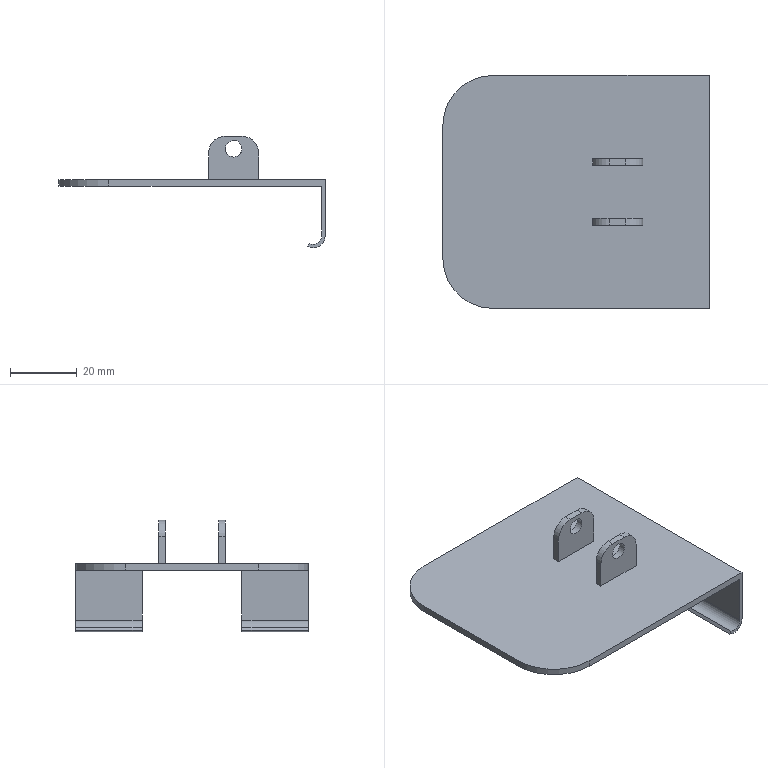Part | NX | features DATUM_CSYS 8, EXTRUDE 7, SKETCH 7, BLEND 2 | 1 solid | 34 faces | box 80 x 70 x 33.5 mm | volume 12516 mm3 | plane 22 | cylinder 12 | commonest cylinder face diameters 5 x4 10 x4 7 x2 30 x2
STEP:
#1=CARTESIAN_POINT('',(22.756,-45.,-24.669));
#2=VERTEX_POINT('',#1);
#3=CARTESIAN_POINT('',(22.756,-25.,-24.669));
#4=VERTEX_POINT('',#3);
#5=CARTESIAN_POINT('',(22.756,-668.,-24.669));
#6=DIRECTION('',(0.,1.,0.));
#7=VECTOR('',#6,1000.);
#8=LINE('',#5,#7);
#9=EDGE_CURVE('',#2,#4,#8,.T.);
#10=ORIENTED_EDGE('',*,*,#9,.T.);
#11=CARTESIAN_POINT('',(22.259,-25.,-25.536));
#12=VERTEX_POINT('',#11);
#13=CARTESIAN_POINT('',(22.756,-25.,-24.669));
#14=DIRECTION('',(-0.4974,0.,-0.8675));
#15=VECTOR('',#14,1000.);
#16=LINE('',#13,#15);
#17=EDGE_CURVE('',#4,#12,#16,.T.);
#18=ORIENTED_EDGE('',*,*,#17,.T.);
#19=CARTESIAN_POINT('',(22.259,-45.,-25.536));
#20=VERTEX_POINT('',#19);
#21=CARTESIAN_POINT('',(22.259,-668.,-25.536));
#22=DIRECTION('',(0.,1.,0.));
#23=VECTOR('',#22,1000.);
#24=LINE('',#21,#23);
#25=EDGE_CURVE('',#20,#12,#24,.T.);
#26=ORIENTED_EDGE('',*,*,#25,.F.);
#27=CARTESIAN_POINT('',(22.756,-45.,-24.669));
#28=DIRECTION('',(-0.4974,0.,-0.8675));
#29=VECTOR('',#28,1000.);
#30=LINE('',#27,#29);
#31=EDGE_CURVE('',#2,#20,#30,.T.);
#32=ORIENTED_EDGE('',*,*,#31,.F.);
#33=EDGE_LOOP('',(#10,#18,#26,#32));
#34=FACE_BOUND('',#33,.T.);
#35=CARTESIAN_POINT('',(22.756,-668.,-24.669));
#36=DIRECTION('',(0.8675,0.,-0.4974));
#37=DIRECTION('',(-0.4974,0.,-0.8675));
#38=AXIS2_PLACEMENT_3D('',#35,#36,#37);
#39=PLANE('',#38);
#40=ADVANCED_FACE('',(#34),#39,.F.);
#41=ORIENTED_EDGE('',*,*,#25,.T.);
#42=CARTESIAN_POINT('',(27.5,-25.,-22.5));
#43=VERTEX_POINT('',#42);
#44=CARTESIAN_POINT('',(24.,-25.,-22.5));
#45=DIRECTION('',(0.,-1.,0.));
#46=DIRECTION('',(0.,0.,-1.));
#47=AXIS2_PLACEMENT_3D('',#44,#45,#46);
#48=CIRCLE('',#47,3.5);
#49=EDGE_CURVE('',#12,#43,#48,.T.);
#50=ORIENTED_EDGE('',*,*,#49,.T.);
#51=CARTESIAN_POINT('',(27.5,-45.,-22.5));
#52=VERTEX_POINT('',#51);
#53=CARTESIAN_POINT('',(27.5,-25.,-22.5));
#54=DIRECTION('',(0.,-1.,0.));
#55=VECTOR('',#54,1000.);
#56=LINE('',#53,#55);
#57=EDGE_CURVE('',#43,#52,#56,.T.);
#58=ORIENTED_EDGE('',*,*,#57,.T.);
#59=CARTESIAN_POINT('',(24.,-45.,-22.5));
#60=DIRECTION('',(0.,-1.,0.));
#61=DIRECTION('',(1.,0.,0.));
#62=AXIS2_PLACEMENT_3D('',#59,#60,#61);
#63=CIRCLE('',#62,3.5);
#64=EDGE_CURVE('',#20,#52,#63,.T.);
#65=ORIENTED_EDGE('',*,*,#64,.F.);
#66=EDGE_LOOP('',(#41,#50,#58,#65));
#67=FACE_BOUND('',#66,.T.);
#68=CARTESIAN_POINT('',(24.,-668.,-22.5));
#69=DIRECTION('',(0.,1.,0.));
#70=DIRECTION('',(-1.,0.,0.));
#71=AXIS2_PLACEMENT_3D('',#68,#69,#70);
#72=CYLINDRICAL_SURFACE('',#71,3.5);
#73=ADVANCED_FACE('',(#67),#72,.T.);
#74=CARTESIAN_POINT('',(26.5,-45.,-22.5));
#75=VERTEX_POINT('',#74);
#76=CARTESIAN_POINT('',(26.5,-25.,-22.5));
#77=VERTEX_POINT('',#76);
#78=CARTESIAN_POINT('',(26.5,-45.,-22.5));
#79=DIRECTION('',(0.,1.,0.));
#80=VECTOR('',#79,1000.);
#81=LINE('',#78,#80);
#82=EDGE_CURVE('',#75,#77,#81,.T.);
#83=ORIENTED_EDGE('',*,*,#82,.T.);
#84=CARTESIAN_POINT('',(24.,-25.,-22.5));
#85=DIRECTION('',(0.,-1.,0.));
#86=DIRECTION('',(0.,0.,-1.));
#87=AXIS2_PLACEMENT_3D('',#84,#85,#86);
#88=CIRCLE('',#87,2.5);
#89=EDGE_CURVE('',#77,#4,#88,.F.);
#90=ORIENTED_EDGE('',*,*,#89,.T.);
#91=ORIENTED_EDGE('',*,*,#9,.F.);
#92=CARTESIAN_POINT('',(24.,-45.,-22.5));
#93=DIRECTION('',(0.,-1.,0.));
#94=DIRECTION('',(1.,0.,0.));
#95=AXIS2_PLACEMENT_3D('',#92,#93,#94);
#96=CIRCLE('',#95,2.5);
#97=EDGE_CURVE('',#75,#2,#96,.F.);
#98=ORIENTED_EDGE('',*,*,#97,.F.);
#99=EDGE_LOOP('',(#83,#90,#91,#98));
#100=FACE_BOUND('',#99,.T.);
#101=CARTESIAN_POINT('',(24.,-668.,-22.5));
#102=DIRECTION('',(0.,1.,0.));
#103=DIRECTION('',(-1.,0.,0.));
#104=AXIS2_PLACEMENT_3D('',#101,#102,#103);
#105=CYLINDRICAL_SURFACE('',#104,2.5);
#106=ADVANCED_FACE('',(#100),#105,.F.);
#107=CARTESIAN_POINT('',(-52.5,-30.,-7.5));
#108=VERTEX_POINT('',#107);
#109=CARTESIAN_POINT('',(-52.5,10.,-7.5));
#110=VERTEX_POINT('',#109);
#111=CARTESIAN_POINT('',(-52.5,-45.,-7.5));
#112=DIRECTION('',(0.,1.,0.));
#113=VECTOR('',#112,1000.);
#114=LINE('',#111,#113);
#115=EDGE_CURVE('',#108,#110,#114,.T.);
#116=ORIENTED_EDGE('',*,*,#115,.T.);
#117=CARTESIAN_POINT('',(-37.5,25.,-7.5));
#118=VERTEX_POINT('',#117);
#119=CARTESIAN_POINT('',(-37.5,10.,-7.5));
#120=DIRECTION('',(0.,0.,1.));
#121=DIRECTION('',(1.,0.,0.));
#122=AXIS2_PLACEMENT_3D('',#119,#120,#121);
#123=CIRCLE('',#122,15.);
#124=EDGE_CURVE('',#110,#118,#123,.F.);
#125=ORIENTED_EDGE('',*,*,#124,.T.);
#126=CARTESIAN_POINT('',(26.5,25.,-7.5));
#127=VERTEX_POINT('',#126);
#128=CARTESIAN_POINT('',(-52.5,25.,-7.5));
#129=DIRECTION('',(1.,0.,0.));
#130=VECTOR('',#129,1000.);
#131=LINE('',#128,#130);
#132=EDGE_CURVE('',#118,#127,#131,.T.);
#133=ORIENTED_EDGE('',*,*,#132,.T.);
#134=CARTESIAN_POINT('',(26.5,5.,-7.5));
#135=VERTEX_POINT('',#134);
#136=CARTESIAN_POINT('',(26.5,5.,-7.5));
#137=DIRECTION('',(0.,1.,0.));
#138=VECTOR('',#137,1000.);
#139=LINE('',#136,#138);
#140=EDGE_CURVE('',#135,#127,#139,.T.);
#141=ORIENTED_EDGE('',*,*,#140,.F.);
#142=CARTESIAN_POINT('',(27.5,5.,-7.5));
#143=VERTEX_POINT('',#142);
#144=CARTESIAN_POINT('',(27.5,5.,-7.5));
#145=DIRECTION('',(-1.,0.,0.));
#146=VECTOR('',#145,1000.);
#147=LINE('',#144,#146);
#148=EDGE_CURVE('',#143,#135,#147,.T.);
#149=ORIENTED_EDGE('',*,*,#148,.F.);
#150=CARTESIAN_POINT('',(27.5,-25.,-7.5));
#151=VERTEX_POINT('',#150);
#152=CARTESIAN_POINT('',(27.5,25.,-7.5));
#153=DIRECTION('',(0.,-1.,0.));
#154=VECTOR('',#153,1000.);
#155=LINE('',#152,#154);
#156=EDGE_CURVE('',#143,#151,#155,.T.);
#157=ORIENTED_EDGE('',*,*,#156,.T.);
#158=CARTESIAN_POINT('',(26.5,-25.,-7.5));
#159=VERTEX_POINT('',#158);
#160=CARTESIAN_POINT('',(26.5,-25.,-7.5));
#161=DIRECTION('',(1.,0.,0.));
#162=VECTOR('',#161,1000.);
#163=LINE('',#160,#162);
#164=EDGE_CURVE('',#159,#151,#163,.T.);
#165=ORIENTED_EDGE('',*,*,#164,.F.);
#166=CARTESIAN_POINT('',(26.5,-45.,-7.5));
#167=VERTEX_POINT('',#166);
#168=CARTESIAN_POINT('',(26.5,-45.,-7.5));
#169=DIRECTION('',(0.,1.,0.));
#170=VECTOR('',#169,1000.);
#171=LINE('',#168,#170);
#172=EDGE_CURVE('',#167,#159,#171,.T.);
#173=ORIENTED_EDGE('',*,*,#172,.F.);
#174=CARTESIAN_POINT('',(-37.5,-45.,-7.5));
#175=VERTEX_POINT('',#174);
#176=CARTESIAN_POINT('',(27.5,-45.,-7.5));
#177=DIRECTION('',(-1.,0.,0.));
#178=VECTOR('',#177,1000.);
#179=LINE('',#176,#178);
#180=EDGE_CURVE('',#167,#175,#179,.T.);
#181=ORIENTED_EDGE('',*,*,#180,.T.);
#182=CARTESIAN_POINT('',(-37.5,-30.,-7.5));
#183=DIRECTION('',(0.,0.,1.));
#184=DIRECTION('',(1.,0.,0.));
#185=AXIS2_PLACEMENT_3D('',#182,#183,#184);
#186=CIRCLE('',#185,15.);
#187=EDGE_CURVE('',#175,#108,#186,.F.);
#188=ORIENTED_EDGE('',*,*,#187,.T.);
#189=EDGE_LOOP('',(#116,#125,#133,#141,#149,#157,#165,#173,#181,#188));
#190=FACE_BOUND('',#189,.T.);
#191=CARTESIAN_POINT('',(-7.5,-20.,-7.5));
#192=DIRECTION('',(0.,0.,1.));
#193=DIRECTION('',(1.,0.,0.));
#194=AXIS2_PLACEMENT_3D('',#191,#192,#193);
#195=PLANE('',#194);
#196=ADVANCED_FACE('',(#190),#195,.F.);
#197=CARTESIAN_POINT('',(-7.5,-20.,2.5));
#198=VERTEX_POINT('',#197);
#199=CARTESIAN_POINT('',(-7.5,-20.,-5.5));
#200=VERTEX_POINT('',#199);
#201=CARTESIAN_POINT('',(-7.5,-20.,7.5));
#202=DIRECTION('',(0.,0.,-1.));
#203=VECTOR('',#202,1000.);
#204=LINE('',#201,#203);
#205=EDGE_CURVE('',#198,#200,#204,.T.);
#206=ORIENTED_EDGE('',*,*,#205,.F.);
#207=CARTESIAN_POINT('',(-7.5,-18.,2.5));
#208=VERTEX_POINT('',#207);
#209=CARTESIAN_POINT('',(-7.5,-20.,2.5));
#210=DIRECTION('',(0.,1.,0.));
#211=VECTOR('',#210,1000.);
#212=LINE('',#209,#211);
#213=EDGE_CURVE('',#198,#208,#212,.T.);
#214=ORIENTED_EDGE('',*,*,#213,.T.);
#215=CARTESIAN_POINT('',(-7.5,-18.,-5.5));
#216=VERTEX_POINT('',#215);
#217=CARTESIAN_POINT('',(-7.5,-18.,7.5));
#218=DIRECTION('',(0.,0.,-1.));
#219=VECTOR('',#218,1000.);
#220=LINE('',#217,#219);
#221=EDGE_CURVE('',#208,#216,#220,.T.);
#222=ORIENTED_EDGE('',*,*,#221,.T.);
#223=CARTESIAN_POINT('',(-7.5,-20.,-5.5));
#224=DIRECTION('',(0.,1.,0.));
#225=VECTOR('',#224,1000.);
#226=LINE('',#223,#225);
#227=EDGE_CURVE('',#216,#200,#226,.F.);
#228=ORIENTED_EDGE('',*,*,#227,.T.);
#229=EDGE_LOOP('',(#206,#214,#222,#228));
#230=FACE_BOUND('',#229,.T.);
#231=CARTESIAN_POINT('',(-7.5,-20.,7.5));
#232=DIRECTION('',(1.,0.,0.));
#233=DIRECTION('',(0.,0.,-1.));
#234=AXIS2_PLACEMENT_3D('',#231,#232,#233);
#235=PLANE('',#234);
#236=ADVANCED_FACE('',(#230),#235,.F.);
#237=CARTESIAN_POINT('',(-7.5,-2.,-5.5));
#238=VERTEX_POINT('',#237);
#239=CARTESIAN_POINT('',(-7.5,-2.,2.5));
#240=VERTEX_POINT('',#239);
#241=CARTESIAN_POINT('',(-7.5,-2.,7.5));
#242=DIRECTION('',(0.,0.,1.));
#243=VECTOR('',#242,1000.);
#244=LINE('',#241,#243);
#245=EDGE_CURVE('',#238,#240,#244,.T.);
#246=ORIENTED_EDGE('',*,*,#245,.T.);
#247=CARTESIAN_POINT('',(-7.5,0.,2.5));
#248=VERTEX_POINT('',#247);
#249=CARTESIAN_POINT('',(-7.5,-20.,2.5));
#250=DIRECTION('',(0.,1.,0.));
#251=VECTOR('',#250,1000.);
#252=LINE('',#249,#251);
#253=EDGE_CURVE('',#240,#248,#252,.T.);
#254=ORIENTED_EDGE('',*,*,#253,.T.);
#255=CARTESIAN_POINT('',(-7.5,0.,-5.5));
#256=VERTEX_POINT('',#255);
#257=CARTESIAN_POINT('',(-7.5,0.,7.5));
#258=DIRECTION('',(0.,0.,-1.));
#259=VECTOR('',#258,1000.);
#260=LINE('',#257,#259);
#261=EDGE_CURVE('',#248,#256,#260,.T.);
#262=ORIENTED_EDGE('',*,*,#261,.T.);
#263=CARTESIAN_POINT('',(-7.5,-20.,-5.5));
#264=DIRECTION('',(0.,1.,0.));
#265=VECTOR('',#264,1000.);
#266=LINE('',#263,#265);
#267=EDGE_CURVE('',#256,#238,#266,.F.);
#268=ORIENTED_EDGE('',*,*,#267,.T.);
#269=EDGE_LOOP('',(#246,#254,#262,#268));
#270=FACE_BOUND('',#269,.T.);
#271=CARTESIAN_POINT('',(-7.5,-20.,7.5));
#272=DIRECTION('',(1.,0.,0.));
#273=DIRECTION('',(0.,0.,-1.));
#274=AXIS2_PLACEMENT_3D('',#271,#272,#273);
#275=PLANE('',#274);
#276=ADVANCED_FACE('',(#270),#275,.F.);
#277=CARTESIAN_POINT('',(7.5,0.,-5.5));
#278=VERTEX_POINT('',#277);
#279=CARTESIAN_POINT('',(7.5,0.,2.5));
#280=VERTEX_POINT('',#279);
#281=CARTESIAN_POINT('',(7.5,0.,-7.5));
#282=DIRECTION('',(0.,0.,1.));
#283=VECTOR('',#282,1000.);
#284=LINE('',#281,#283);
#285=EDGE_CURVE('',#278,#280,#284,.T.);
#286=ORIENTED_EDGE('',*,*,#285,.T.);
#287=CARTESIAN_POINT('',(7.5,-2.,2.5));
#288=VERTEX_POINT('',#287);
#289=CARTESIAN_POINT('',(7.5,-20.,2.5));
#290=DIRECTION('',(0.,1.,0.));
#291=VECTOR('',#290,1000.);
#292=LINE('',#289,#291);
#293=EDGE_CURVE('',#280,#288,#292,.F.);
#294=ORIENTED_EDGE('',*,*,#293,.T.);
#295=CARTESIAN_POINT('',(7.5,-2.,-5.5));
#296=VERTEX_POINT('',#295);
#297=CARTESIAN_POINT('',(7.5,-2.,-7.5));
#298=DIRECTION('',(0.,0.,-1.));
#299=VECTOR('',#298,1000.);
#300=LINE('',#297,#299);
#301=EDGE_CURVE('',#288,#296,#300,.T.);
#302=ORIENTED_EDGE('',*,*,#301,.T.);
#303=CARTESIAN_POINT('',(7.5,-20.,-5.5));
#304=DIRECTION('',(0.,-1.,0.));
#305=VECTOR('',#304,1000.);
#306=LINE('',#303,#305);
#307=EDGE_CURVE('',#296,#278,#306,.F.);
#308=ORIENTED_EDGE('',*,*,#307,.T.);
#309=EDGE_LOOP('',(#286,#294,#302,#308));
#310=FACE_BOUND('',#309,.T.);
#311=CARTESIAN_POINT('',(7.5,-20.,-7.5));
#312=DIRECTION('',(-1.,0.,0.));
#313=DIRECTION('',(0.,0.,1.));
#314=AXIS2_PLACEMENT_3D('',#311,#312,#313);
#315=PLANE('',#314);
#316=ADVANCED_FACE('',(#310),#315,.F.);
#317=CARTESIAN_POINT('',(7.5,-18.,-5.5));
#318=VERTEX_POINT('',#317);
#319=CARTESIAN_POINT('',(7.5,-18.,2.5));
#320=VERTEX_POINT('',#319);
#321=CARTESIAN_POINT('',(7.5,-18.,-7.5));
#322=DIRECTION('',(0.,0.,1.));
#323=VECTOR('',#322,1000.);
#324=LINE('',#321,#323);
#325=EDGE_CURVE('',#318,#320,#324,.T.);
#326=ORIENTED_EDGE('',*,*,#325,.T.);
#327=CARTESIAN_POINT('',(7.5,-20.,2.5));
#328=VERTEX_POINT('',#327);
#329=CARTESIAN_POINT('',(7.5,-20.,2.5));
#330=DIRECTION('',(0.,1.,0.));
#331=VECTOR('',#330,1000.);
#332=LINE('',#329,#331);
#333=EDGE_CURVE('',#320,#328,#332,.F.);
#334=ORIENTED_EDGE('',*,*,#333,.T.);
#335=CARTESIAN_POINT('',(7.5,-20.,-5.5));
#336=VERTEX_POINT('',#335);
#337=CARTESIAN_POINT('',(7.5,-20.,-7.5));
#338=DIRECTION('',(0.,0.,1.));
#339=VECTOR('',#338,1000.);
#340=LINE('',#337,#339);
#341=EDGE_CURVE('',#336,#328,#340,.T.);
#342=ORIENTED_EDGE('',*,*,#341,.F.);
#343=CARTESIAN_POINT('',(7.5,-20.,-5.5));
#344=DIRECTION('',(0.,-1.,0.));
#345=VECTOR('',#344,1000.);
#346=LINE('',#343,#345);
#347=EDGE_CURVE('',#336,#318,#346,.F.);
#348=ORIENTED_EDGE('',*,*,#347,.T.);
#349=EDGE_LOOP('',(#326,#334,#342,#348));
#350=FACE_BOUND('',#349,.T.);
#351=CARTESIAN_POINT('',(7.5,-20.,-7.5));
#352=DIRECTION('',(-1.,0.,0.));
#353=DIRECTION('',(0.,0.,1.));
#354=AXIS2_PLACEMENT_3D('',#351,#352,#353);
#355=PLANE('',#354);
#356=ADVANCED_FACE('',(#350),#355,.F.);
#357=CARTESIAN_POINT('',(0.,-20.,1.25));
#358=VERTEX_POINT('',#357);
#359=CARTESIAN_POINT('',(0.,-20.,3.75));
#360=DIRECTION('',(0.,-1.,0.));
#361=DIRECTION('',(0.,0.,-1.));
#362=AXIS2_PLACEMENT_3D('',#359,#360,#361);
#363=CIRCLE('',#362,2.5);
#364=EDGE_CURVE('',#358,#358,#363,.T.);
#365=ORIENTED_EDGE('',*,*,#364,.F.);
#366=EDGE_LOOP('',(#365));
#367=FACE_BOUND('',#366,.T.);
#368=CARTESIAN_POINT('',(2.5,-20.,7.5));
#369=VERTEX_POINT('',#368);
#370=CARTESIAN_POINT('',(-2.5,-20.,7.5));
#371=VERTEX_POINT('',#370);
#372=CARTESIAN_POINT('',(7.5,-20.,7.5));
#373=DIRECTION('',(-1.,0.,0.));
#374=VECTOR('',#373,1000.);
#375=LINE('',#372,#374);
#376=EDGE_CURVE('',#369,#371,#375,.T.);
#377=ORIENTED_EDGE('',*,*,#376,.T.);
#378=CARTESIAN_POINT('',(-2.5,-20.,2.5));
#379=DIRECTION('',(0.,-1.,0.));
#380=DIRECTION('',(0.,0.,-1.));
#381=AXIS2_PLACEMENT_3D('',#378,#379,#380);
#382=CIRCLE('',#381,5.);
#383=EDGE_CURVE('',#371,#198,#382,.T.);
#384=ORIENTED_EDGE('',*,*,#383,.T.);
#385=ORIENTED_EDGE('',*,*,#205,.T.);
#386=CARTESIAN_POINT('',(0.,-20.,-5.5));
#387=DIRECTION('',(1.,0.,0.));
#388=VECTOR('',#387,1000.);
#389=LINE('',#386,#388);
#390=EDGE_CURVE('',#200,#336,#389,.T.);
#391=ORIENTED_EDGE('',*,*,#390,.T.);
#392=ORIENTED_EDGE('',*,*,#341,.T.);
#393=CARTESIAN_POINT('',(2.5,-20.,2.5));
#394=DIRECTION('',(0.,-1.,0.));
#395=DIRECTION('',(0.,0.,-1.));
#396=AXIS2_PLACEMENT_3D('',#393,#394,#395);
#397=CIRCLE('',#396,5.);
#398=EDGE_CURVE('',#328,#369,#397,.T.);
#399=ORIENTED_EDGE('',*,*,#398,.T.);
#400=EDGE_LOOP('',(#377,#384,#385,#391,#392,#399));
#401=FACE_BOUND('',#400,.T.);
#402=CARTESIAN_POINT('',(0.,-20.,0.));
#403=DIRECTION('',(0.,-1.,0.));
#404=DIRECTION('',(0.,0.,-1.));
#405=AXIS2_PLACEMENT_3D('',#402,#403,#404);
#406=PLANE('',#405);
#407=ADVANCED_FACE('',(#367,#401),#406,.T.);
#408=CARTESIAN_POINT('',(-2.5,0.,3.75));
#409=VERTEX_POINT('',#408);
#410=CARTESIAN_POINT('',(0.,0.,3.75));
#411=DIRECTION('',(0.,1.,0.));
#412=DIRECTION('',(-1.,0.,0.));
#413=AXIS2_PLACEMENT_3D('',#410,#411,#412);
#414=CIRCLE('',#413,2.5);
#415=EDGE_CURVE('',#409,#409,#414,.T.);
#416=ORIENTED_EDGE('',*,*,#415,.F.);
#417=EDGE_LOOP('',(#416));
#418=FACE_BOUND('',#417,.T.);
#419=CARTESIAN_POINT('',(2.5,0.,7.5));
#420=VERTEX_POINT('',#419);
#421=CARTESIAN_POINT('',(-2.5,0.,7.5));
#422=VERTEX_POINT('',#421);
#423=CARTESIAN_POINT('',(7.5,0.,7.5));
#424=DIRECTION('',(-1.,0.,0.));
#425=VECTOR('',#424,1000.);
#426=LINE('',#423,#425);
#427=EDGE_CURVE('',#420,#422,#426,.T.);
#428=ORIENTED_EDGE('',*,*,#427,.F.);
#429=CARTESIAN_POINT('',(2.5,0.,2.5));
#430=DIRECTION('',(0.,-1.,0.));
#431=DIRECTION('',(0.,0.,-1.));
#432=AXIS2_PLACEMENT_3D('',#429,#430,#431);
#433=CIRCLE('',#432,5.);
#434=EDGE_CURVE('',#420,#280,#433,.F.);
#435=ORIENTED_EDGE('',*,*,#434,.T.);
#436=ORIENTED_EDGE('',*,*,#285,.F.);
#437=CARTESIAN_POINT('',(0.,0.,-5.5));
#438=DIRECTION('',(1.,0.,0.));
#439=VECTOR('',#438,1000.);
#440=LINE('',#437,#439);
#441=EDGE_CURVE('',#256,#278,#440,.T.);
#442=ORIENTED_EDGE('',*,*,#441,.F.);
#443=ORIENTED_EDGE('',*,*,#261,.F.);
#444=CARTESIAN_POINT('',(-2.5,0.,2.5));
#445=DIRECTION('',(0.,-1.,0.));
#446=DIRECTION('',(0.,0.,-1.));
#447=AXIS2_PLACEMENT_3D('',#444,#445,#446);
#448=CIRCLE('',#447,5.);
#449=EDGE_CURVE('',#248,#422,#448,.F.);
#450=ORIENTED_EDGE('',*,*,#449,.T.);
#451=EDGE_LOOP('',(#428,#435,#436,#442,#443,#450));
#452=FACE_BOUND('',#451,.T.);
#453=CARTESIAN_POINT('',(0.,0.,0.));
#454=DIRECTION('',(0.,-1.,0.));
#455=DIRECTION('',(0.,0.,-1.));
#456=AXIS2_PLACEMENT_3D('',#453,#454,#455);
#457=PLANE('',#456);
#458=ADVANCED_FACE('',(#418,#452),#457,.F.);
#459=CARTESIAN_POINT('',(-2.5,-2.,7.5));
#460=VERTEX_POINT('',#459);
#461=CARTESIAN_POINT('',(2.5,-2.,7.5));
#462=VERTEX_POINT('',#461);
#463=CARTESIAN_POINT('',(7.5,-2.,7.5));
#464=DIRECTION('',(1.,0.,0.));
#465=VECTOR('',#464,1000.);
#466=LINE('',#463,#465);
#467=EDGE_CURVE('',#460,#462,#466,.T.);
#468=ORIENTED_EDGE('',*,*,#467,.T.);
#469=CARTESIAN_POINT('',(2.5,-20.,7.5));
#470=DIRECTION('',(0.,1.,0.));
#471=VECTOR('',#470,1000.);
#472=LINE('',#469,#471);
#473=EDGE_CURVE('',#462,#420,#472,.T.);
#474=ORIENTED_EDGE('',*,*,#473,.T.);
#475=ORIENTED_EDGE('',*,*,#427,.T.);
#476=CARTESIAN_POINT('',(-2.5,-20.,7.5));
#477=DIRECTION('',(0.,1.,0.));
#478=VECTOR('',#477,1000.);
#479=LINE('',#476,#478);
#480=EDGE_CURVE('',#422,#460,#479,.F.);
#481=ORIENTED_EDGE('',*,*,#480,.T.);
#482=EDGE_LOOP('',(#468,#474,#475,#481));
#483=FACE_BOUND('',#482,.T.);
#484=CARTESIAN_POINT('',(7.5,-20.,7.5));
#485=DIRECTION('',(0.,0.,-1.));
#486=DIRECTION('',(-1.,0.,0.));
#487=AXIS2_PLACEMENT_3D('',#484,#485,#486);
#488=PLANE('',#487);
#489=ADVANCED_FACE('',(#483),#488,.F.);
#490=CARTESIAN_POINT('',(2.5,-18.,7.5));
#491=VERTEX_POINT('',#490);
#492=CARTESIAN_POINT('',(-2.5,-18.,7.5));
#493=VERTEX_POINT('',#492);
#494=CARTESIAN_POINT('',(7.5,-18.,7.5));
#495=DIRECTION('',(-1.,0.,0.));
#496=VECTOR('',#495,1000.);
#497=LINE('',#494,#496);
#498=EDGE_CURVE('',#491,#493,#497,.T.);
#499=ORIENTED_EDGE('',*,*,#498,.T.);
#500=CARTESIAN_POINT('',(-2.5,-20.,7.5));
#501=DIRECTION('',(0.,1.,0.));
#502=VECTOR('',#501,1000.);
#503=LINE('',#500,#502);
#504=EDGE_CURVE('',#493,#371,#503,.F.);
#505=ORIENTED_EDGE('',*,*,#504,.T.);
#506=ORIENTED_EDGE('',*,*,#376,.F.);
#507=CARTESIAN_POINT('',(2.5,-20.,7.5));
#508=DIRECTION('',(0.,1.,0.));
#509=VECTOR('',#508,1000.);
#510=LINE('',#507,#509);
#511=EDGE_CURVE('',#369,#491,#510,.T.);
#512=ORIENTED_EDGE('',*,*,#511,.T.);
#513=EDGE_LOOP('',(#499,#505,#506,#512));
#514=FACE_BOUND('',#513,.T.);
#515=CARTESIAN_POINT('',(7.5,-20.,7.5));
#516=DIRECTION('',(0.,0.,-1.));
#517=DIRECTION('',(-1.,0.,0.));
#518=AXIS2_PLACEMENT_3D('',#515,#516,#517);
#519=PLANE('',#518);
#520=ADVANCED_FACE('',(#514),#519,.F.);
#521=CARTESIAN_POINT('',(-23.,-2.,-5.5));
#522=DIRECTION('',(1.,0.,0.));
#523=VECTOR('',#522,1000.);
#524=LINE('',#521,#523);
#525=EDGE_CURVE('',#296,#238,#524,.F.);
#526=ORIENTED_EDGE('',*,*,#525,.T.);
#527=ORIENTED_EDGE('',*,*,#267,.F.);
#528=ORIENTED_EDGE('',*,*,#441,.T.);
#529=ORIENTED_EDGE('',*,*,#307,.F.);
#530=EDGE_LOOP('',(#526,#527,#528,#529));
#531=FACE_BOUND('',#530,.T.);
#532=CARTESIAN_POINT('',(21.,-18.,-5.5));
#533=DIRECTION('',(-1.,0.,0.));
#534=VECTOR('',#533,1000.);
#535=LINE('',#532,#534);
#536=EDGE_CURVE('',#216,#318,#535,.F.);
#537=ORIENTED_EDGE('',*,*,#536,.T.);
#538=ORIENTED_EDGE('',*,*,#347,.F.);
#539=ORIENTED_EDGE('',*,*,#390,.F.);
#540=ORIENTED_EDGE('',*,*,#227,.F.);
#541=EDGE_LOOP('',(#537,#538,#539,#540));
#542=FACE_BOUND('',#541,.T.);
#543=CARTESIAN_POINT('',(-37.5,25.,-5.5));
#544=VERTEX_POINT('',#543);
#545=CARTESIAN_POINT('',(27.5,25.,-5.5));
#546=VERTEX_POINT('',#545);
#547=CARTESIAN_POINT('',(-52.5,25.,-5.5));
#548=DIRECTION('',(1.,0.,0.));
#549=VECTOR('',#548,1000.);
#550=LINE('',#547,#549);
#551=EDGE_CURVE('',#544,#546,#550,.T.);
#552=ORIENTED_EDGE('',*,*,#551,.F.);
#553=CARTESIAN_POINT('',(-52.5,10.,-5.5));
#554=VERTEX_POINT('',#553);
#555=CARTESIAN_POINT('',(-37.5,10.,-5.5));
#556=DIRECTION('',(0.,0.,-1.));
#557=DIRECTION('',(-1.,0.,0.));
#558=AXIS2_PLACEMENT_3D('',#555,#556,#557);
#559=CIRCLE('',#558,15.);
#560=EDGE_CURVE('',#544,#554,#559,.F.);
#561=ORIENTED_EDGE('',*,*,#560,.T.);
#562=CARTESIAN_POINT('',(-52.5,-30.,-5.5));
#563=VERTEX_POINT('',#562);
#564=CARTESIAN_POINT('',(-52.5,-45.,-5.5));
#565=DIRECTION('',(0.,1.,0.));
#566=VECTOR('',#565,1000.);
#567=LINE('',#564,#566);
#568=EDGE_CURVE('',#563,#554,#567,.T.);
#569=ORIENTED_EDGE('',*,*,#568,.F.);
#570=CARTESIAN_POINT('',(-37.5,-45.,-5.5));
#571=VERTEX_POINT('',#570);
#572=CARTESIAN_POINT('',(-37.5,-30.,-5.5));
#573=DIRECTION('',(0.,0.,-1.));
#574=DIRECTION('',(-1.,0.,0.));
#575=AXIS2_PLACEMENT_3D('',#572,#573,#574);
#576=CIRCLE('',#575,15.);
#577=EDGE_CURVE('',#563,#571,#576,.F.);
#578=ORIENTED_EDGE('',*,*,#577,.T.);
#579=CARTESIAN_POINT('',(27.5,-45.,-5.5));
#580=VERTEX_POINT('',#579);
#581=CARTESIAN_POINT('',(27.5,-45.,-5.5));
#582=DIRECTION('',(-1.,0.,0.));
#583=VECTOR('',#582,1000.);
#584=LINE('',#581,#583);
#585=EDGE_CURVE('',#580,#571,#584,.T.);
#586=ORIENTED_EDGE('',*,*,#585,.F.);
#587=CARTESIAN_POINT('',(27.5,25.,-5.5));
#588=DIRECTION('',(0.,-1.,0.));
#589=VECTOR('',#588,1000.);
#590=LINE('',#587,#589);
#591=EDGE_CURVE('',#546,#580,#590,.T.);
#592=ORIENTED_EDGE('',*,*,#591,.F.);
#593=EDGE_LOOP('',(#552,#561,#569,#578,#586,#592));
#594=FACE_BOUND('',#593,.T.);
#595=CARTESIAN_POINT('',(0.,0.,-5.5));
#596=DIRECTION('',(0.,0.,-1.));
#597=DIRECTION('',(-1.,0.,0.));
#598=AXIS2_PLACEMENT_3D('',#595,#596,#597);
#599=PLANE('',#598);
#600=ADVANCED_FACE('',(#531,#542,#594),#599,.F.);
#601=CARTESIAN_POINT('',(-2.5,-2.,3.75));
#602=VERTEX_POINT('',#601);
#603=CARTESIAN_POINT('',(0.,-2.,3.75));
#604=DIRECTION('',(0.,1.,0.));
#605=DIRECTION('',(-1.,0.,0.));
#606=AXIS2_PLACEMENT_3D('',#603,#604,#605);
#607=CIRCLE('',#606,2.5);
#608=EDGE_CURVE('',#602,#602,#607,.T.);
#609=ORIENTED_EDGE('',*,*,#608,.T.);
#610=EDGE_LOOP('',(#609));
#611=FACE_BOUND('',#610,.T.);
#612=ORIENTED_EDGE('',*,*,#301,.F.);
#613=CARTESIAN_POINT('',(2.5,-2.,2.5));
#614=DIRECTION('',(0.,1.,0.));
#615=DIRECTION('',(-1.,0.,0.));
#616=AXIS2_PLACEMENT_3D('',#613,#614,#615);
#617=CIRCLE('',#616,5.);
#618=EDGE_CURVE('',#288,#462,#617,.F.);
#619=ORIENTED_EDGE('',*,*,#618,.T.);
#620=ORIENTED_EDGE('',*,*,#467,.F.);
#621=CARTESIAN_POINT('',(-2.5,-2.,2.5));
#622=DIRECTION('',(0.,1.,0.));
#623=DIRECTION('',(-1.,0.,0.));
#624=AXIS2_PLACEMENT_3D('',#621,#622,#623);
#625=CIRCLE('',#624,5.);
#626=EDGE_CURVE('',#460,#240,#625,.F.);
#627=ORIENTED_EDGE('',*,*,#626,.T.);
#628=ORIENTED_EDGE('',*,*,#245,.F.);
#629=ORIENTED_EDGE('',*,*,#525,.F.);
#630=EDGE_LOOP('',(#612,#619,#620,#627,#628,#629));
#631=FACE_BOUND('',#630,.T.);
#632=CARTESIAN_POINT('',(-23.,-2.,10.5));
#633=DIRECTION('',(0.,1.,0.));
#634=DIRECTION('',(-1.,0.,0.));
#635=AXIS2_PLACEMENT_3D('',#632,#633,#634);
#636=PLANE('',#635);
#637=ADVANCED_FACE('',(#611,#631),#636,.F.);
#638=CARTESIAN_POINT('',(2.5,-18.,3.75));
#639=VERTEX_POINT('',#638);
#640=CARTESIAN_POINT('',(0.,-18.,3.75));
#641=DIRECTION('',(0.,-1.,0.));
#642=DIRECTION('',(1.,0.,0.));
#643=AXIS2_PLACEMENT_3D('',#640,#641,#642);
#644=CIRCLE('',#643,2.5);
#645=EDGE_CURVE('',#639,#639,#644,.T.);
#646=ORIENTED_EDGE('',*,*,#645,.T.);
#647=EDGE_LOOP('',(#646));
#648=FACE_BOUND('',#647,.T.);
#649=ORIENTED_EDGE('',*,*,#221,.F.);
#650=CARTESIAN_POINT('',(-2.5,-18.,2.5));
#651=DIRECTION('',(0.,-1.,0.));
#652=DIRECTION('',(1.,0.,0.));
#653=AXIS2_PLACEMENT_3D('',#650,#651,#652);
#654=CIRCLE('',#653,5.);
#655=EDGE_CURVE('',#208,#493,#654,.F.);
#656=ORIENTED_EDGE('',*,*,#655,.T.);
#657=ORIENTED_EDGE('',*,*,#498,.F.);
#658=CARTESIAN_POINT('',(2.5,-18.,2.5));
#659=DIRECTION('',(0.,-1.,0.));
#660=DIRECTION('',(1.,0.,0.));
#661=AXIS2_PLACEMENT_3D('',#658,#659,#660);
#662=CIRCLE('',#661,5.);
#663=EDGE_CURVE('',#491,#320,#662,.F.);
#664=ORIENTED_EDGE('',*,*,#663,.T.);
#665=ORIENTED_EDGE('',*,*,#325,.F.);
#666=ORIENTED_EDGE('',*,*,#536,.F.);
#667=EDGE_LOOP('',(#649,#656,#657,#664,#665,#666));
#668=FACE_BOUND('',#667,.T.);
#669=CARTESIAN_POINT('',(21.,-18.,10.5));
#670=DIRECTION('',(0.,-1.,0.));
#671=DIRECTION('',(1.,0.,0.));
#672=AXIS2_PLACEMENT_3D('',#669,#670,#671);
#673=PLANE('',#672);
#674=ADVANCED_FACE('',(#648,#668),#673,.F.);
#675=ORIENTED_EDGE('',*,*,#568,.T.);
#676=CARTESIAN_POINT('',(-52.5,10.,-5.5));
#677=DIRECTION('',(0.,0.,-1.));
#678=VECTOR('',#677,1000.);
#679=LINE('',#676,#678);
#680=EDGE_CURVE('',#554,#110,#679,.T.);
#681=ORIENTED_EDGE('',*,*,#680,.T.);
#682=ORIENTED_EDGE('',*,*,#115,.F.);
#683=CARTESIAN_POINT('',(-52.5,-30.,-5.5));
#684=DIRECTION('',(0.,0.,-1.));
#685=VECTOR('',#684,1000.);
#686=LINE('',#683,#685);
#687=EDGE_CURVE('',#108,#563,#686,.F.);
#688=ORIENTED_EDGE('',*,*,#687,.T.);
#689=EDGE_LOOP('',(#675,#681,#682,#688));
#690=FACE_BOUND('',#689,.T.);
#691=CARTESIAN_POINT('',(-52.5,-45.,-5.5));
#692=DIRECTION('',(-1.,0.,0.));
#693=DIRECTION('',(0.,-1.,0.));
#694=AXIS2_PLACEMENT_3D('',#691,#692,#693);
#695=PLANE('',#694);
#696=ADVANCED_FACE('',(#690),#695,.T.);
#697=ORIENTED_EDGE('',*,*,#132,.F.);
#698=CARTESIAN_POINT('',(-37.5,25.,-5.5));
#699=DIRECTION('',(0.,0.,-1.));
#700=VECTOR('',#699,1000.);
#701=LINE('',#698,#700);
#702=EDGE_CURVE('',#118,#544,#701,.F.);
#703=ORIENTED_EDGE('',*,*,#702,.T.);
#704=ORIENTED_EDGE('',*,*,#551,.T.);
#705=CARTESIAN_POINT('',(27.5,25.,-22.5));
#706=VERTEX_POINT('',#705);
#707=CARTESIAN_POINT('',(27.5,25.,-5.5));
#708=DIRECTION('',(0.,0.,-1.));
#709=VECTOR('',#708,1000.);
#710=LINE('',#707,#709);
#711=EDGE_CURVE('',#546,#706,#710,.T.);
#712=ORIENTED_EDGE('',*,*,#711,.T.);
#713=CARTESIAN_POINT('',(22.259,25.,-25.536));
#714=VERTEX_POINT('',#713);
#715=CARTESIAN_POINT('',(24.,25.,-22.5));
#716=DIRECTION('',(0.,-1.,0.));
#717=DIRECTION('',(0.,0.,-1.));
#718=AXIS2_PLACEMENT_3D('',#715,#716,#717);
#719=CIRCLE('',#718,3.5);
#720=EDGE_CURVE('',#714,#706,#719,.T.);
#721=ORIENTED_EDGE('',*,*,#720,.F.);
#722=CARTESIAN_POINT('',(22.756,25.,-24.669));
#723=VERTEX_POINT('',#722);
#724=CARTESIAN_POINT('',(22.756,25.,-24.669));
#725=DIRECTION('',(-0.4974,0.,-0.8675));
#726=VECTOR('',#725,1000.);
#727=LINE('',#724,#726);
#728=EDGE_CURVE('',#723,#714,#727,.T.);
#729=ORIENTED_EDGE('',*,*,#728,.F.);
#730=CARTESIAN_POINT('',(26.5,25.,-22.5));
#731=VERTEX_POINT('',#730);
#732=CARTESIAN_POINT('',(24.,25.,-22.5));
#733=DIRECTION('',(0.,1.,0.));
#734=DIRECTION('',(0.,0.,-1.));
#735=AXIS2_PLACEMENT_3D('',#732,#733,#734);
#736=CIRCLE('',#735,2.5);
#737=EDGE_CURVE('',#731,#723,#736,.T.);
#738=ORIENTED_EDGE('',*,*,#737,.F.);
#739=CARTESIAN_POINT('',(26.5,25.,-22.5));
#740=DIRECTION('',(0.,0.,1.));
#741=VECTOR('',#740,1000.);
#742=LINE('',#739,#741);
#743=EDGE_CURVE('',#731,#127,#742,.T.);
#744=ORIENTED_EDGE('',*,*,#743,.T.);
#745=EDGE_LOOP('',(#697,#703,#704,#712,#721,#729,#738,#744));
#746=FACE_BOUND('',#745,.T.);
#747=CARTESIAN_POINT('',(-52.5,25.,-5.5));
#748=DIRECTION('',(0.,1.,0.));
#749=DIRECTION('',(-1.,0.,0.));
#750=AXIS2_PLACEMENT_3D('',#747,#748,#749);
#751=PLANE('',#750);
#752=ADVANCED_FACE('',(#746),#751,.T.);
#753=ORIENTED_EDGE('',*,*,#156,.F.);
#754=CARTESIAN_POINT('',(27.5,5.,-22.5));
#755=VERTEX_POINT('',#754);
#756=CARTESIAN_POINT('',(27.5,5.,-22.5));
#757=DIRECTION('',(0.,0.,1.));
#758=VECTOR('',#757,1000.);
#759=LINE('',#756,#758);
#760=EDGE_CURVE('',#755,#143,#759,.T.);
#761=ORIENTED_EDGE('',*,*,#760,.F.);
#762=CARTESIAN_POINT('',(27.5,25.,-22.5));
#763=DIRECTION('',(0.,-1.,0.));
#764=VECTOR('',#763,1000.);
#765=LINE('',#762,#764);
#766=EDGE_CURVE('',#706,#755,#765,.T.);
#767=ORIENTED_EDGE('',*,*,#766,.F.);
#768=ORIENTED_EDGE('',*,*,#711,.F.);
#769=ORIENTED_EDGE('',*,*,#591,.T.);
#770=CARTESIAN_POINT('',(27.5,-45.,-5.5));
#771=DIRECTION('',(0.,0.,-1.));
#772=VECTOR('',#771,1000.);
#773=LINE('',#770,#772);
#774=EDGE_CURVE('',#580,#52,#773,.T.);
#775=ORIENTED_EDGE('',*,*,#774,.T.);
#776=ORIENTED_EDGE('',*,*,#57,.F.);
#777=CARTESIAN_POINT('',(27.5,-25.,-22.5));
#778=DIRECTION('',(0.,0.,1.));
#779=VECTOR('',#778,1000.);
#780=LINE('',#777,#779);
#781=EDGE_CURVE('',#43,#151,#780,.T.);
#782=ORIENTED_EDGE('',*,*,#781,.T.);
#783=EDGE_LOOP('',(#753,#761,#767,#768,#769,#775,#776,#782));
#784=FACE_BOUND('',#783,.T.);
#785=CARTESIAN_POINT('',(27.5,25.,-5.5));
#786=DIRECTION('',(1.,0.,0.));
#787=DIRECTION('',(0.,1.,0.));
#788=AXIS2_PLACEMENT_3D('',#785,#786,#787);
#789=PLANE('',#788);
#790=ADVANCED_FACE('',(#784),#789,.T.);
#791=ORIENTED_EDGE('',*,*,#585,.T.);
#792=CARTESIAN_POINT('',(-37.5,-45.,-5.5));
#793=DIRECTION('',(0.,0.,-1.));
#794=VECTOR('',#793,1000.);
#795=LINE('',#792,#794);
#796=EDGE_CURVE('',#571,#175,#795,.T.);
#797=ORIENTED_EDGE('',*,*,#796,.T.);
#798=ORIENTED_EDGE('',*,*,#180,.F.);
#799=CARTESIAN_POINT('',(26.5,-45.,-22.5));
#800=DIRECTION('',(0.,0.,1.));
#801=VECTOR('',#800,1000.);
#802=LINE('',#799,#801);
#803=EDGE_CURVE('',#75,#167,#802,.T.);
#804=ORIENTED_EDGE('',*,*,#803,.F.);
#805=ORIENTED_EDGE('',*,*,#97,.T.);
#806=ORIENTED_EDGE('',*,*,#31,.T.);
#807=ORIENTED_EDGE('',*,*,#64,.T.);
#808=ORIENTED_EDGE('',*,*,#774,.F.);
#809=EDGE_LOOP('',(#791,#797,#798,#804,#805,#806,#807,#808));
#810=FACE_BOUND('',#809,.T.);
#811=CARTESIAN_POINT('',(27.5,-45.,-5.5));
#812=DIRECTION('',(0.,-1.,0.));
#813=DIRECTION('',(1.,0.,0.));
#814=AXIS2_PLACEMENT_3D('',#811,#812,#813);
#815=PLANE('',#814);
#816=ADVANCED_FACE('',(#810),#815,.T.);
#817=ORIENTED_EDGE('',*,*,#172,.T.);
#818=CARTESIAN_POINT('',(26.5,-25.,-22.5));
#819=DIRECTION('',(0.,0.,1.));
#820=VECTOR('',#819,1000.);
#821=LINE('',#818,#820);
#822=EDGE_CURVE('',#77,#159,#821,.T.);
#823=ORIENTED_EDGE('',*,*,#822,.F.);
#824=ORIENTED_EDGE('',*,*,#82,.F.);
#825=ORIENTED_EDGE('',*,*,#803,.T.);
#826=EDGE_LOOP('',(#817,#823,#824,#825));
#827=FACE_BOUND('',#826,.T.);
#828=CARTESIAN_POINT('',(26.5,-45.,-22.5));
#829=DIRECTION('',(1.,0.,0.));
#830=DIRECTION('',(0.,1.,0.));
#831=AXIS2_PLACEMENT_3D('',#828,#829,#830);
#832=PLANE('',#831);
#833=ADVANCED_FACE('',(#827),#832,.F.);
#834=ORIENTED_EDGE('',*,*,#164,.T.);
#835=ORIENTED_EDGE('',*,*,#781,.F.);
#836=ORIENTED_EDGE('',*,*,#49,.F.);
#837=ORIENTED_EDGE('',*,*,#17,.F.);
#838=ORIENTED_EDGE('',*,*,#89,.F.);
#839=ORIENTED_EDGE('',*,*,#822,.T.);
#840=EDGE_LOOP('',(#834,#835,#836,#837,#838,#839));
#841=FACE_BOUND('',#840,.T.);
#842=CARTESIAN_POINT('',(26.5,-25.,-22.5));
#843=DIRECTION('',(0.,-1.,0.));
#844=DIRECTION('',(1.,0.,0.));
#845=AXIS2_PLACEMENT_3D('',#842,#843,#844);
#846=PLANE('',#845);
#847=ADVANCED_FACE('',(#841),#846,.F.);
#848=ORIENTED_EDGE('',*,*,#140,.T.);
#849=ORIENTED_EDGE('',*,*,#743,.F.);
#850=CARTESIAN_POINT('',(26.5,5.,-22.5));
#851=VERTEX_POINT('',#850);
#852=CARTESIAN_POINT('',(26.5,5.,-22.5));
#853=DIRECTION('',(0.,1.,0.));
#854=VECTOR('',#853,1000.);
#855=LINE('',#852,#854);
#856=EDGE_CURVE('',#851,#731,#855,.T.);
#857=ORIENTED_EDGE('',*,*,#856,.F.);
#858=CARTESIAN_POINT('',(26.5,5.,-22.5));
#859=DIRECTION('',(0.,0.,1.));
#860=VECTOR('',#859,1000.);
#861=LINE('',#858,#860);
#862=EDGE_CURVE('',#851,#135,#861,.T.);
#863=ORIENTED_EDGE('',*,*,#862,.T.);
#864=EDGE_LOOP('',(#848,#849,#857,#863));
#865=FACE_BOUND('',#864,.T.);
#866=CARTESIAN_POINT('',(26.5,5.,-22.5));
#867=DIRECTION('',(1.,0.,0.));
#868=DIRECTION('',(0.,1.,0.));
#869=AXIS2_PLACEMENT_3D('',#866,#867,#868);
#870=PLANE('',#869);
#871=ADVANCED_FACE('',(#865),#870,.F.);
#872=ORIENTED_EDGE('',*,*,#148,.T.);
#873=ORIENTED_EDGE('',*,*,#862,.F.);
#874=CARTESIAN_POINT('',(22.756,5.,-24.669));
#875=VERTEX_POINT('',#874);
#876=CARTESIAN_POINT('',(24.,5.,-22.5));
#877=DIRECTION('',(0.,1.,0.));
#878=DIRECTION('',(0.,0.,1.));
#879=AXIS2_PLACEMENT_3D('',#876,#877,#878);
#880=CIRCLE('',#879,2.5);
#881=EDGE_CURVE('',#875,#851,#880,.F.);
#882=ORIENTED_EDGE('',*,*,#881,.F.);
#883=CARTESIAN_POINT('',(22.259,5.,-25.536));
#884=VERTEX_POINT('',#883);
#885=CARTESIAN_POINT('',(22.756,5.,-24.669));
#886=DIRECTION('',(0.4974,0.,0.8675));
#887=VECTOR('',#886,1000.);
#888=LINE('',#885,#887);
#889=EDGE_CURVE('',#884,#875,#888,.T.);
#890=ORIENTED_EDGE('',*,*,#889,.F.);
#891=CARTESIAN_POINT('',(24.,5.,-22.5));
#892=DIRECTION('',(0.,1.,0.));
#893=DIRECTION('',(0.,0.,1.));
#894=AXIS2_PLACEMENT_3D('',#891,#892,#893);
#895=CIRCLE('',#894,3.5);
#896=EDGE_CURVE('',#755,#884,#895,.T.);
#897=ORIENTED_EDGE('',*,*,#896,.F.);
#898=ORIENTED_EDGE('',*,*,#760,.T.);
#899=EDGE_LOOP('',(#872,#873,#882,#890,#897,#898));
#900=FACE_BOUND('',#899,.T.);
#901=CARTESIAN_POINT('',(27.5,5.,-22.5));
#902=DIRECTION('',(0.,1.,0.));
#903=DIRECTION('',(-1.,0.,0.));
#904=AXIS2_PLACEMENT_3D('',#901,#902,#903);
#905=PLANE('',#904);
#906=ADVANCED_FACE('',(#900),#905,.F.);
#907=CARTESIAN_POINT('',(22.259,-668.,-25.536));
#908=DIRECTION('',(0.,1.,0.));
#909=VECTOR('',#908,1000.);
#910=LINE('',#907,#909);
#911=EDGE_CURVE('',#884,#714,#910,.T.);
#912=ORIENTED_EDGE('',*,*,#911,.F.);
#913=ORIENTED_EDGE('',*,*,#889,.T.);
#914=CARTESIAN_POINT('',(22.756,-668.,-24.669));
#915=DIRECTION('',(0.,1.,0.));
#916=VECTOR('',#915,1000.);
#917=LINE('',#914,#916);
#918=EDGE_CURVE('',#875,#723,#917,.T.);
#919=ORIENTED_EDGE('',*,*,#918,.T.);
#920=ORIENTED_EDGE('',*,*,#728,.T.);
#921=EDGE_LOOP('',(#912,#913,#919,#920));
#922=FACE_BOUND('',#921,.T.);
#923=CARTESIAN_POINT('',(22.756,-668.,-24.669));
#924=DIRECTION('',(0.8675,0.,-0.4974));
#925=DIRECTION('',(-0.4974,0.,-0.8675));
#926=AXIS2_PLACEMENT_3D('',#923,#924,#925);
#927=PLANE('',#926);
#928=ADVANCED_FACE('',(#922),#927,.F.);
#929=ORIENTED_EDGE('',*,*,#766,.T.);
#930=ORIENTED_EDGE('',*,*,#896,.T.);
#931=ORIENTED_EDGE('',*,*,#911,.T.);
#932=ORIENTED_EDGE('',*,*,#720,.T.);
#933=EDGE_LOOP('',(#929,#930,#931,#932));
#934=FACE_BOUND('',#933,.T.);
#935=CARTESIAN_POINT('',(24.,-668.,-22.5));
#936=DIRECTION('',(0.,1.,0.));
#937=DIRECTION('',(-1.,0.,0.));
#938=AXIS2_PLACEMENT_3D('',#935,#936,#937);
#939=CYLINDRICAL_SURFACE('',#938,3.5);
#940=ADVANCED_FACE('',(#934),#939,.T.);
#941=ORIENTED_EDGE('',*,*,#918,.F.);
#942=ORIENTED_EDGE('',*,*,#881,.T.);
#943=ORIENTED_EDGE('',*,*,#856,.T.);
#944=ORIENTED_EDGE('',*,*,#737,.T.);
#945=EDGE_LOOP('',(#941,#942,#943,#944));
#946=FACE_BOUND('',#945,.T.);
#947=CARTESIAN_POINT('',(24.,-668.,-22.5));
#948=DIRECTION('',(0.,1.,0.));
#949=DIRECTION('',(-1.,0.,0.));
#950=AXIS2_PLACEMENT_3D('',#947,#948,#949);
#951=CYLINDRICAL_SURFACE('',#950,2.5);
#952=ADVANCED_FACE('',(#946),#951,.F.);
#953=ORIENTED_EDGE('',*,*,#560,.F.);
#954=ORIENTED_EDGE('',*,*,#702,.F.);
#955=ORIENTED_EDGE('',*,*,#124,.F.);
#956=ORIENTED_EDGE('',*,*,#680,.F.);
#957=EDGE_LOOP('',(#953,#954,#955,#956));
#958=FACE_BOUND('',#957,.T.);
#959=CARTESIAN_POINT('',(-37.5,10.,-5.5));
#960=DIRECTION('',(0.,0.,-1.));
#961=DIRECTION('',(-1.,0.,0.));
#962=AXIS2_PLACEMENT_3D('',#959,#960,#961);
#963=CYLINDRICAL_SURFACE('',#962,15.);
#964=ADVANCED_FACE('',(#958),#963,.T.);
#965=ORIENTED_EDGE('',*,*,#577,.F.);
#966=ORIENTED_EDGE('',*,*,#687,.F.);
#967=ORIENTED_EDGE('',*,*,#187,.F.);
#968=ORIENTED_EDGE('',*,*,#796,.F.);
#969=EDGE_LOOP('',(#965,#966,#967,#968));
#970=FACE_BOUND('',#969,.T.);
#971=CARTESIAN_POINT('',(-37.5,-30.,-5.5));
#972=DIRECTION('',(0.,0.,-1.));
#973=DIRECTION('',(-1.,0.,0.));
#974=AXIS2_PLACEMENT_3D('',#971,#972,#973);
#975=CYLINDRICAL_SURFACE('',#974,15.);
#976=ADVANCED_FACE('',(#970),#975,.T.);
#977=ORIENTED_EDGE('',*,*,#364,.T.);
#978=EDGE_LOOP('',(#977));
#979=FACE_BOUND('',#978,.T.);
#980=ORIENTED_EDGE('',*,*,#645,.F.);
#981=EDGE_LOOP('',(#980));
#982=FACE_BOUND('',#981,.T.);
#983=CARTESIAN_POINT('',(0.,-53.,3.75));
#984=DIRECTION('',(0.,1.,0.));
#985=DIRECTION('',(0.,0.,1.));
#986=AXIS2_PLACEMENT_3D('',#983,#984,#985);
#987=CYLINDRICAL_SURFACE('',#986,2.5);
#988=ADVANCED_FACE('',(#979,#982),#987,.F.);
#989=ORIENTED_EDGE('',*,*,#415,.T.);
#990=EDGE_LOOP('',(#989));
#991=FACE_BOUND('',#990,.T.);
#992=ORIENTED_EDGE('',*,*,#608,.F.);
#993=EDGE_LOOP('',(#992));
#994=FACE_BOUND('',#993,.T.);
#995=CARTESIAN_POINT('',(0.,-53.,3.75));
#996=DIRECTION('',(0.,1.,0.));
#997=DIRECTION('',(0.,0.,1.));
#998=AXIS2_PLACEMENT_3D('',#995,#996,#997);
#999=CYLINDRICAL_SURFACE('',#998,2.5);
#1000=ADVANCED_FACE('',(#991,#994),#999,.F.);
#1001=ORIENTED_EDGE('',*,*,#618,.F.);
#1002=ORIENTED_EDGE('',*,*,#293,.F.);
#1003=ORIENTED_EDGE('',*,*,#434,.F.);
#1004=ORIENTED_EDGE('',*,*,#473,.F.);
#1005=EDGE_LOOP('',(#1001,#1002,#1003,#1004));
#1006=FACE_BOUND('',#1005,.T.);
#1007=CARTESIAN_POINT('',(2.5,-20.,2.5));
#1008=DIRECTION('',(0.,1.,0.));
#1009=DIRECTION('',(0.,0.,1.));
#1010=AXIS2_PLACEMENT_3D('',#1007,#1008,#1009);
#1011=CYLINDRICAL_SURFACE('',#1010,5.);
#1012=ADVANCED_FACE('',(#1006),#1011,.T.);
#1013=ORIENTED_EDGE('',*,*,#626,.F.);
#1014=ORIENTED_EDGE('',*,*,#480,.F.);
#1015=ORIENTED_EDGE('',*,*,#449,.F.);
#1016=ORIENTED_EDGE('',*,*,#253,.F.);
#1017=EDGE_LOOP('',(#1013,#1014,#1015,#1016));
#1018=FACE_BOUND('',#1017,.T.);
#1019=CARTESIAN_POINT('',(-2.5,-20.,2.5));
#1020=DIRECTION('',(0.,1.,0.));
#1021=DIRECTION('',(0.,0.,1.));
#1022=AXIS2_PLACEMENT_3D('',#1019,#1020,#1021);
#1023=CYLINDRICAL_SURFACE('',#1022,5.);
#1024=ADVANCED_FACE('',(#1018),#1023,.T.);
#1025=ORIENTED_EDGE('',*,*,#383,.F.);
#1026=ORIENTED_EDGE('',*,*,#504,.F.);
#1027=ORIENTED_EDGE('',*,*,#655,.F.);
#1028=ORIENTED_EDGE('',*,*,#213,.F.);
#1029=EDGE_LOOP('',(#1025,#1026,#1027,#1028));
#1030=FACE_BOUND('',#1029,.T.);
#1031=CARTESIAN_POINT('',(-2.5,-20.,2.5));
#1032=DIRECTION('',(0.,1.,0.));
#1033=DIRECTION('',(0.,0.,1.));
#1034=AXIS2_PLACEMENT_3D('',#1031,#1032,#1033);
#1035=CYLINDRICAL_SURFACE('',#1034,5.);
#1036=ADVANCED_FACE('',(#1030),#1035,.T.);
#1037=ORIENTED_EDGE('',*,*,#398,.F.);
#1038=ORIENTED_EDGE('',*,*,#333,.F.);
#1039=ORIENTED_EDGE('',*,*,#663,.F.);
#1040=ORIENTED_EDGE('',*,*,#511,.F.);
#1041=EDGE_LOOP('',(#1037,#1038,#1039,#1040));
#1042=FACE_BOUND('',#1041,.T.);
#1043=CARTESIAN_POINT('',(2.5,-20.,2.5));
#1044=DIRECTION('',(0.,1.,0.));
#1045=DIRECTION('',(0.,0.,1.));
#1046=AXIS2_PLACEMENT_3D('',#1043,#1044,#1045);
#1047=CYLINDRICAL_SURFACE('',#1046,5.);
#1048=ADVANCED_FACE('',(#1042),#1047,.T.);
#1049=CLOSED_SHELL('',(#40,#73,#106,#196,#236,#276,#316,#356,#407,#458,#489,#520,#600,#637,#674,#696,#752,#790,#816,#833,#847,#871,#906,#928,#940,#952,#964,#976,#988,#1000,#1012,#1024,#1036,#1048));
#1050=MANIFOLD_SOLID_BREP('',#1049);
#1051=(LENGTH_UNIT()NAMED_UNIT(*)SI_UNIT(.MILLI.,.METRE.));
#1052=UNCERTAINTY_MEASURE_WITH_UNIT(LENGTH_MEASURE(0.00001),#1051,'','');
#1053=(NAMED_UNIT(*)PLANE_ANGLE_UNIT()SI_UNIT($,.RADIAN.));
#1054=(NAMED_UNIT(*)SI_UNIT($,.STERADIAN.)SOLID_ANGLE_UNIT());
#1055=(GEOMETRIC_REPRESENTATION_CONTEXT(3)GLOBAL_UNCERTAINTY_ASSIGNED_CONTEXT((#1052))GLOBAL_UNIT_ASSIGNED_CONTEXT((#1051,#1053,#1054))REPRESENTATION_CONTEXT('',''));
#1056=ADVANCED_BREP_SHAPE_REPRESENTATION('',(#1050),#1055);